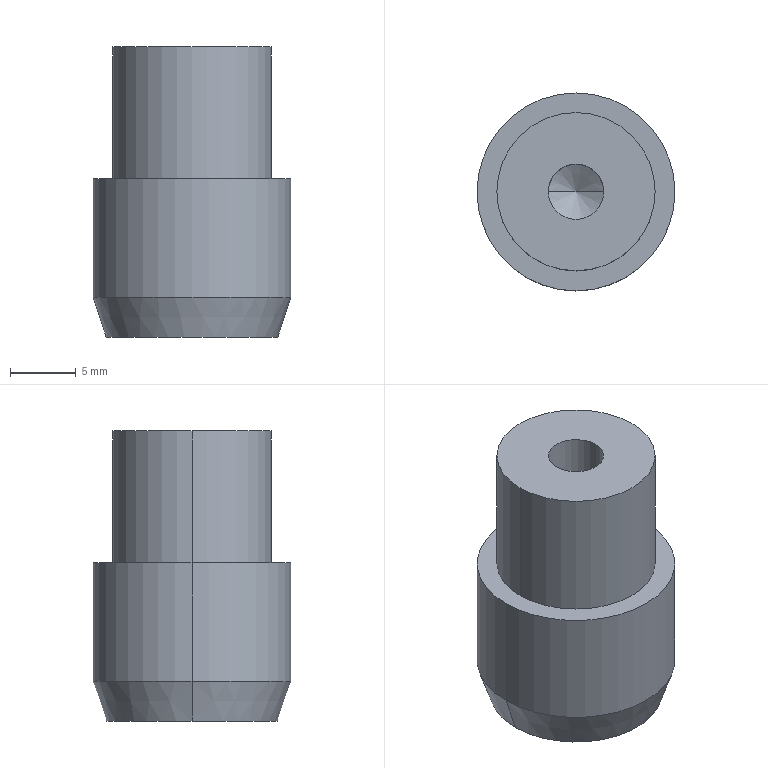Part | NX | features BREP 1 | 1 solid | 13 faces | box 15 x 15 x 22 mm | volume 3006 mm3 | cylinder 6 | cone 4 | plane 3 | commonest cylinder face diameters 4.2 x2 12 x2 15 x2
STEP:
#1=CARTESIAN_POINT('',(-174.167,-108.703,9.6));
#2=VERTEX_POINT('',#1);
#3=CARTESIAN_POINT('',(-169.967,-108.703,9.6));
#4=VERTEX_POINT('',#3);
#5=CARTESIAN_POINT('',(-172.067,-108.703,9.6));
#6=DIRECTION('',(0.,0.,1.));
#7=DIRECTION('',(1.,0.,0.));
#8=AXIS2_PLACEMENT_3D('',#5,#6,#7);
#9=CIRCLE('',#8,2.1);
#10=EDGE_CURVE('',#2,#4,#9,.T.);
#11=ORIENTED_EDGE('',*,*,#10,.F.);
#12=CARTESIAN_POINT('',(-174.167,-108.703,22.));
#13=VERTEX_POINT('',#12);
#14=CARTESIAN_POINT('',(-174.167,-108.703,22.));
#15=DIRECTION('',(0.,0.,1.));
#16=VECTOR('',#15,1000.);
#17=LINE('',#14,#16);
#18=EDGE_CURVE('',#13,#2,#17,.F.);
#19=ORIENTED_EDGE('',*,*,#18,.F.);
#20=CARTESIAN_POINT('',(-169.967,-108.703,22.));
#21=VERTEX_POINT('',#20);
#22=CARTESIAN_POINT('',(-172.067,-108.703,22.));
#23=DIRECTION('',(0.,0.,1.));
#24=DIRECTION('',(1.,0.,0.));
#25=AXIS2_PLACEMENT_3D('',#22,#23,#24);
#26=CIRCLE('',#25,2.1);
#27=EDGE_CURVE('',#13,#21,#26,.T.);
#28=ORIENTED_EDGE('',*,*,#27,.T.);
#29=CARTESIAN_POINT('',(-169.967,-108.703,22.));
#30=DIRECTION('',(0.,0.,1.));
#31=VECTOR('',#30,1000.);
#32=LINE('',#29,#31);
#33=EDGE_CURVE('',#21,#4,#32,.F.);
#34=ORIENTED_EDGE('',*,*,#33,.T.);
#35=EDGE_LOOP('',(#11,#19,#28,#34));
#36=FACE_BOUND('',#35,.T.);
#37=CARTESIAN_POINT('',(-172.067,-108.703,22.));
#38=DIRECTION('',(0.,0.,1.));
#39=DIRECTION('',(1.,0.,0.));
#40=AXIS2_PLACEMENT_3D('',#37,#38,#39);
#41=CYLINDRICAL_SURFACE('',#40,2.1);
#42=ADVANCED_FACE('',(#36),#41,.F.);
#43=CARTESIAN_POINT('',(-172.067,-108.703,8.338));
#44=VERTEX_POINT('',#43);
#45=CARTESIAN_POINT('',(-169.967,-108.703,9.6));
#46=DIRECTION('',(0.8572,0.,0.515));
#47=VECTOR('',#46,1000.);
#48=LINE('',#45,#47);
#49=EDGE_CURVE('',#4,#44,#48,.F.);
#50=ORIENTED_EDGE('',*,*,#49,.T.);
#51=CARTESIAN_POINT('',(-174.167,-108.703,9.6));
#52=DIRECTION('',(-0.8572,0.,0.515));
#53=VECTOR('',#52,1000.);
#54=LINE('',#51,#53);
#55=EDGE_CURVE('',#2,#44,#54,.F.);
#56=ORIENTED_EDGE('',*,*,#55,.F.);
#57=ORIENTED_EDGE('',*,*,#10,.T.);
#58=EDGE_LOOP('',(#50,#56,#57));
#59=FACE_BOUND('',#58,.T.);
#60=CARTESIAN_POINT('',(-172.067,-108.703,9.6));
#61=DIRECTION('',(0.,0.,1.));
#62=DIRECTION('',(1.,0.,0.));
#63=AXIS2_PLACEMENT_3D('',#60,#61,#62);
#64=CONICAL_SURFACE('',#63,2.1,1.03);
#65=ADVANCED_FACE('',(#59),#64,.F.);
#66=CARTESIAN_POINT('',(-178.567,-108.703,0.));
#67=VERTEX_POINT('',#66);
#68=CARTESIAN_POINT('',(-165.567,-108.703,0.));
#69=VERTEX_POINT('',#68);
#70=CARTESIAN_POINT('',(-172.067,-108.703,0.));
#71=DIRECTION('',(0.,0.,-1.));
#72=DIRECTION('',(1.,0.,0.));
#73=AXIS2_PLACEMENT_3D('',#70,#71,#72);
#74=CIRCLE('',#73,6.5);
#75=EDGE_CURVE('',#67,#69,#74,.T.);
#76=ORIENTED_EDGE('',*,*,#75,.F.);
#77=CARTESIAN_POINT('',(-179.567,-108.703,3.));
#78=VERTEX_POINT('',#77);
#79=CARTESIAN_POINT('',(-179.567,-108.703,3.));
#80=DIRECTION('',(-0.3162,0.,0.9487));
#81=VECTOR('',#80,1000.);
#82=LINE('',#79,#81);
#83=EDGE_CURVE('',#78,#67,#82,.F.);
#84=ORIENTED_EDGE('',*,*,#83,.F.);
#85=CARTESIAN_POINT('',(-164.567,-108.703,3.));
#86=VERTEX_POINT('',#85);
#87=CARTESIAN_POINT('',(-172.067,-108.703,3.));
#88=DIRECTION('',(0.,0.,1.));
#89=DIRECTION('',(1.,0.,0.));
#90=AXIS2_PLACEMENT_3D('',#87,#88,#89);
#91=CIRCLE('',#90,7.5);
#92=EDGE_CURVE('',#86,#78,#91,.T.);
#93=ORIENTED_EDGE('',*,*,#92,.F.);
#94=CARTESIAN_POINT('',(-164.567,-108.703,3.));
#95=DIRECTION('',(0.3162,0.,0.9487));
#96=VECTOR('',#95,1000.);
#97=LINE('',#94,#96);
#98=EDGE_CURVE('',#86,#69,#97,.F.);
#99=ORIENTED_EDGE('',*,*,#98,.T.);
#100=EDGE_LOOP('',(#76,#84,#93,#99));
#101=FACE_BOUND('',#100,.T.);
#102=CARTESIAN_POINT('',(-172.067,-108.703,3.));
#103=DIRECTION('',(0.,0.,1.));
#104=DIRECTION('',(1.,0.,0.));
#105=AXIS2_PLACEMENT_3D('',#102,#103,#104);
#106=CONICAL_SURFACE('',#105,7.5,0.3218);
#107=ADVANCED_FACE('',(#101),#106,.T.);
#108=CARTESIAN_POINT('',(-166.067,-108.703,22.));
#109=VERTEX_POINT('',#108);
#110=CARTESIAN_POINT('',(-178.067,-108.703,22.));
#111=VERTEX_POINT('',#110);
#112=CARTESIAN_POINT('',(-172.067,-108.703,22.));
#113=DIRECTION('',(0.,0.,1.));
#114=DIRECTION('',(1.,0.,0.));
#115=AXIS2_PLACEMENT_3D('',#112,#113,#114);
#116=CIRCLE('',#115,6.);
#117=EDGE_CURVE('',#109,#111,#116,.T.);
#118=ORIENTED_EDGE('',*,*,#117,.F.);
#119=CARTESIAN_POINT('',(-166.067,-108.703,12.));
#120=VERTEX_POINT('',#119);
#121=CARTESIAN_POINT('',(-166.067,-108.703,22.));
#122=DIRECTION('',(0.,0.,-1.));
#123=VECTOR('',#122,1000.);
#124=LINE('',#121,#123);
#125=EDGE_CURVE('',#109,#120,#124,.T.);
#126=ORIENTED_EDGE('',*,*,#125,.T.);
#127=CARTESIAN_POINT('',(-178.067,-108.703,12.));
#128=VERTEX_POINT('',#127);
#129=CARTESIAN_POINT('',(-172.067,-108.703,12.));
#130=DIRECTION('',(0.,0.,1.));
#131=DIRECTION('',(1.,0.,0.));
#132=AXIS2_PLACEMENT_3D('',#129,#130,#131);
#133=CIRCLE('',#132,6.);
#134=EDGE_CURVE('',#120,#128,#133,.T.);
#135=ORIENTED_EDGE('',*,*,#134,.T.);
#136=CARTESIAN_POINT('',(-178.067,-108.703,22.));
#137=DIRECTION('',(0.,0.,-1.));
#138=VECTOR('',#137,1000.);
#139=LINE('',#136,#138);
#140=EDGE_CURVE('',#111,#128,#139,.T.);
#141=ORIENTED_EDGE('',*,*,#140,.F.);
#142=EDGE_LOOP('',(#118,#126,#135,#141));
#143=FACE_BOUND('',#142,.T.);
#144=CARTESIAN_POINT('',(-172.067,-108.703,22.));
#145=DIRECTION('',(0.,0.,-1.));
#146=DIRECTION('',(-1.,0.,0.));
#147=AXIS2_PLACEMENT_3D('',#144,#145,#146);
#148=CYLINDRICAL_SURFACE('',#147,6.);
#149=ADVANCED_FACE('',(#143),#148,.T.);
#150=CARTESIAN_POINT('',(-164.567,-108.703,12.));
#151=VERTEX_POINT('',#150);
#152=CARTESIAN_POINT('',(-179.567,-108.703,12.));
#153=VERTEX_POINT('',#152);
#154=CARTESIAN_POINT('',(-172.067,-108.703,12.));
#155=DIRECTION('',(0.,0.,1.));
#156=DIRECTION('',(1.,0.,0.));
#157=AXIS2_PLACEMENT_3D('',#154,#155,#156);
#158=CIRCLE('',#157,7.5);
#159=EDGE_CURVE('',#151,#153,#158,.T.);
#160=ORIENTED_EDGE('',*,*,#159,.F.);
#161=CARTESIAN_POINT('',(-164.567,-108.703,12.));
#162=DIRECTION('',(0.,0.,-1.));
#163=VECTOR('',#162,1000.);
#164=LINE('',#161,#163);
#165=EDGE_CURVE('',#151,#86,#164,.T.);
#166=ORIENTED_EDGE('',*,*,#165,.T.);
#167=ORIENTED_EDGE('',*,*,#92,.T.);
#168=CARTESIAN_POINT('',(-179.567,-108.703,12.));
#169=DIRECTION('',(0.,0.,-1.));
#170=VECTOR('',#169,1000.);
#171=LINE('',#168,#170);
#172=EDGE_CURVE('',#153,#78,#171,.T.);
#173=ORIENTED_EDGE('',*,*,#172,.F.);
#174=EDGE_LOOP('',(#160,#166,#167,#173));
#175=FACE_BOUND('',#174,.T.);
#176=CARTESIAN_POINT('',(-172.067,-108.703,12.));
#177=DIRECTION('',(0.,0.,-1.));
#178=DIRECTION('',(-1.,0.,0.));
#179=AXIS2_PLACEMENT_3D('',#176,#177,#178);
#180=CYLINDRICAL_SURFACE('',#179,7.5);
#181=ADVANCED_FACE('',(#175),#180,.T.);
#182=CARTESIAN_POINT('',(-172.067,-108.703,12.));
#183=DIRECTION('',(0.,0.,1.));
#184=DIRECTION('',(1.,0.,0.));
#185=AXIS2_PLACEMENT_3D('',#182,#183,#184);
#186=CIRCLE('',#185,7.5);
#187=EDGE_CURVE('',#153,#151,#186,.T.);
#188=ORIENTED_EDGE('',*,*,#187,.T.);
#189=ORIENTED_EDGE('',*,*,#159,.T.);
#190=EDGE_LOOP('',(#188,#189));
#191=FACE_BOUND('',#190,.T.);
#192=CARTESIAN_POINT('',(-172.067,-108.703,12.));
#193=DIRECTION('',(0.,0.,1.));
#194=DIRECTION('',(1.,0.,0.));
#195=AXIS2_PLACEMENT_3D('',#192,#193,#194);
#196=CIRCLE('',#195,6.);
#197=EDGE_CURVE('',#128,#120,#196,.T.);
#198=ORIENTED_EDGE('',*,*,#197,.F.);
#199=ORIENTED_EDGE('',*,*,#134,.F.);
#200=EDGE_LOOP('',(#198,#199));
#201=FACE_BOUND('',#200,.T.);
#202=CARTESIAN_POINT('',(-172.067,-108.703,12.));
#203=DIRECTION('',(0.,0.,1.));
#204=DIRECTION('',(1.,0.,0.));
#205=AXIS2_PLACEMENT_3D('',#202,#203,#204);
#206=PLANE('',#205);
#207=ADVANCED_FACE('',(#191,#201),#206,.T.);
#208=ORIENTED_EDGE('',*,*,#165,.F.);
#209=ORIENTED_EDGE('',*,*,#187,.F.);
#210=ORIENTED_EDGE('',*,*,#172,.T.);
#211=CARTESIAN_POINT('',(-172.067,-108.703,3.));
#212=DIRECTION('',(0.,0.,1.));
#213=DIRECTION('',(1.,0.,0.));
#214=AXIS2_PLACEMENT_3D('',#211,#212,#213);
#215=CIRCLE('',#214,7.5);
#216=EDGE_CURVE('',#78,#86,#215,.T.);
#217=ORIENTED_EDGE('',*,*,#216,.T.);
#218=EDGE_LOOP('',(#208,#209,#210,#217));
#219=FACE_BOUND('',#218,.T.);
#220=CARTESIAN_POINT('',(-172.067,-108.703,12.));
#221=DIRECTION('',(0.,0.,-1.));
#222=DIRECTION('',(-1.,0.,0.));
#223=AXIS2_PLACEMENT_3D('',#220,#221,#222);
#224=CYLINDRICAL_SURFACE('',#223,7.5);
#225=ADVANCED_FACE('',(#219),#224,.T.);
#226=CARTESIAN_POINT('',(-172.067,-108.703,0.));
#227=DIRECTION('',(0.,0.,-1.));
#228=DIRECTION('',(1.,0.,0.));
#229=AXIS2_PLACEMENT_3D('',#226,#227,#228);
#230=CIRCLE('',#229,6.5);
#231=EDGE_CURVE('',#69,#67,#230,.T.);
#232=ORIENTED_EDGE('',*,*,#231,.T.);
#233=ORIENTED_EDGE('',*,*,#75,.T.);
#234=EDGE_LOOP('',(#232,#233));
#235=FACE_BOUND('',#234,.T.);
#236=CARTESIAN_POINT('',(-172.067,-108.703,0.));
#237=DIRECTION('',(0.,0.,1.));
#238=DIRECTION('',(1.,0.,0.));
#239=AXIS2_PLACEMENT_3D('',#236,#237,#238);
#240=PLANE('',#239);
#241=ADVANCED_FACE('',(#235),#240,.F.);
#242=ORIENTED_EDGE('',*,*,#125,.F.);
#243=CARTESIAN_POINT('',(-172.067,-108.703,22.));
#244=DIRECTION('',(0.,0.,1.));
#245=DIRECTION('',(1.,0.,0.));
#246=AXIS2_PLACEMENT_3D('',#243,#244,#245);
#247=CIRCLE('',#246,6.);
#248=EDGE_CURVE('',#111,#109,#247,.T.);
#249=ORIENTED_EDGE('',*,*,#248,.F.);
#250=ORIENTED_EDGE('',*,*,#140,.T.);
#251=ORIENTED_EDGE('',*,*,#197,.T.);
#252=EDGE_LOOP('',(#242,#249,#250,#251));
#253=FACE_BOUND('',#252,.T.);
#254=CARTESIAN_POINT('',(-172.067,-108.703,22.));
#255=DIRECTION('',(0.,0.,-1.));
#256=DIRECTION('',(-1.,0.,0.));
#257=AXIS2_PLACEMENT_3D('',#254,#255,#256);
#258=CYLINDRICAL_SURFACE('',#257,6.);
#259=ADVANCED_FACE('',(#253),#258,.T.);
#260=ORIENTED_EDGE('',*,*,#248,.T.);
#261=ORIENTED_EDGE('',*,*,#117,.T.);
#262=EDGE_LOOP('',(#260,#261));
#263=FACE_BOUND('',#262,.T.);
#264=CARTESIAN_POINT('',(-172.067,-108.703,22.));
#265=DIRECTION('',(0.,0.,1.));
#266=DIRECTION('',(1.,0.,0.));
#267=AXIS2_PLACEMENT_3D('',#264,#265,#266);
#268=CIRCLE('',#267,2.1);
#269=EDGE_CURVE('',#21,#13,#268,.T.);
#270=ORIENTED_EDGE('',*,*,#269,.F.);
#271=ORIENTED_EDGE('',*,*,#27,.F.);
#272=EDGE_LOOP('',(#270,#271));
#273=FACE_BOUND('',#272,.T.);
#274=CARTESIAN_POINT('',(-172.067,-108.703,22.));
#275=DIRECTION('',(0.,0.,1.));
#276=DIRECTION('',(1.,0.,0.));
#277=AXIS2_PLACEMENT_3D('',#274,#275,#276);
#278=PLANE('',#277);
#279=ADVANCED_FACE('',(#263,#273),#278,.T.);
#280=ORIENTED_EDGE('',*,*,#83,.T.);
#281=ORIENTED_EDGE('',*,*,#231,.F.);
#282=ORIENTED_EDGE('',*,*,#98,.F.);
#283=ORIENTED_EDGE('',*,*,#216,.F.);
#284=EDGE_LOOP('',(#280,#281,#282,#283));
#285=FACE_BOUND('',#284,.T.);
#286=CARTESIAN_POINT('',(-172.067,-108.703,3.));
#287=DIRECTION('',(0.,0.,1.));
#288=DIRECTION('',(1.,0.,0.));
#289=AXIS2_PLACEMENT_3D('',#286,#287,#288);
#290=CONICAL_SURFACE('',#289,7.5,0.3218);
#291=ADVANCED_FACE('',(#285),#290,.T.);
#292=ORIENTED_EDGE('',*,*,#55,.T.);
#293=ORIENTED_EDGE('',*,*,#49,.F.);
#294=CARTESIAN_POINT('',(-172.067,-108.703,9.6));
#295=DIRECTION('',(0.,0.,1.));
#296=DIRECTION('',(1.,0.,0.));
#297=AXIS2_PLACEMENT_3D('',#294,#295,#296);
#298=CIRCLE('',#297,2.1);
#299=EDGE_CURVE('',#4,#2,#298,.T.);
#300=ORIENTED_EDGE('',*,*,#299,.T.);
#301=EDGE_LOOP('',(#292,#293,#300));
#302=FACE_BOUND('',#301,.T.);
#303=CARTESIAN_POINT('',(-172.067,-108.703,9.6));
#304=DIRECTION('',(0.,0.,1.));
#305=DIRECTION('',(1.,0.,0.));
#306=AXIS2_PLACEMENT_3D('',#303,#304,#305);
#307=CONICAL_SURFACE('',#306,2.1,1.03);
#308=ADVANCED_FACE('',(#302),#307,.F.);
#309=ORIENTED_EDGE('',*,*,#18,.T.);
#310=ORIENTED_EDGE('',*,*,#299,.F.);
#311=ORIENTED_EDGE('',*,*,#33,.F.);
#312=ORIENTED_EDGE('',*,*,#269,.T.);
#313=EDGE_LOOP('',(#309,#310,#311,#312));
#314=FACE_BOUND('',#313,.T.);
#315=CARTESIAN_POINT('',(-172.067,-108.703,22.));
#316=DIRECTION('',(0.,0.,1.));
#317=DIRECTION('',(1.,0.,0.));
#318=AXIS2_PLACEMENT_3D('',#315,#316,#317);
#319=CYLINDRICAL_SURFACE('',#318,2.1);
#320=ADVANCED_FACE('',(#314),#319,.F.);
#321=CLOSED_SHELL('',(#42,#65,#107,#149,#181,#207,#225,#241,#259,#279,#291,#308,#320));
#322=MANIFOLD_SOLID_BREP('',#321);
#323=(LENGTH_UNIT()NAMED_UNIT(*)SI_UNIT(.MILLI.,.METRE.));
#324=UNCERTAINTY_MEASURE_WITH_UNIT(LENGTH_MEASURE(0.00001),#323,'','');
#325=(NAMED_UNIT(*)PLANE_ANGLE_UNIT()SI_UNIT($,.RADIAN.));
#326=(NAMED_UNIT(*)SI_UNIT($,.STERADIAN.)SOLID_ANGLE_UNIT());
#327=(GEOMETRIC_REPRESENTATION_CONTEXT(3)GLOBAL_UNCERTAINTY_ASSIGNED_CONTEXT((#324))GLOBAL_UNIT_ASSIGNED_CONTEXT((#323,#325,#326))REPRESENTATION_CONTEXT('',''));
#328=ADVANCED_BREP_SHAPE_REPRESENTATION('',(#322),#327);